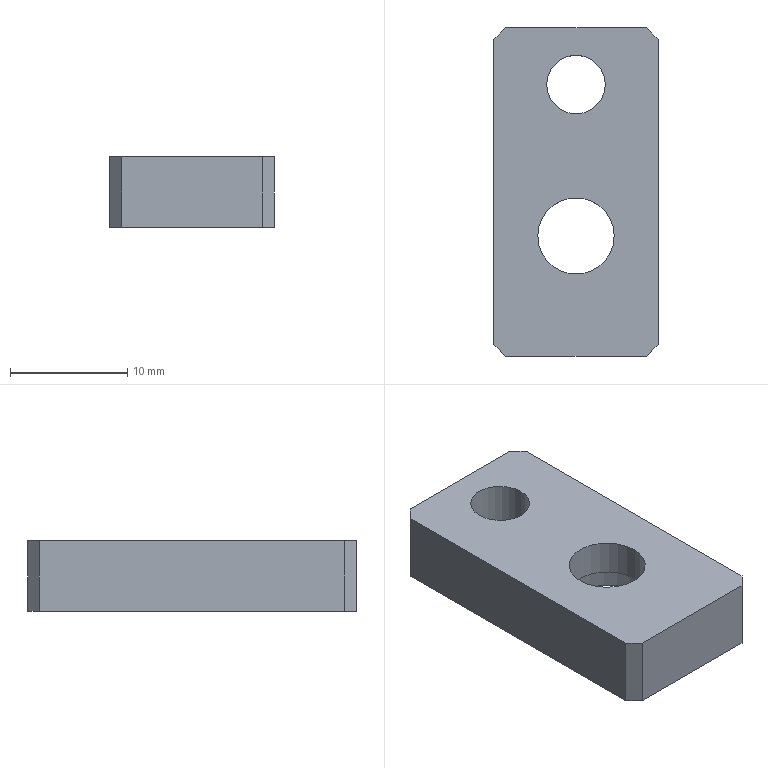Part | STEP file | Front Guide Wheel Fixing Plate | 1 solid | 17 faces | box 14 x 28 x 6 mm | volume 1838 mm3 | plane 11 | cylinder 6 | commonest cylinder face diameters 5 x2 6.5 x2 11 x2
STEP:
#1=CARTESIAN_POINT('',(0.,0.,0.));
#2=DIRECTION('',(0.,0.,1.));
#3=DIRECTION('',(1.,0.,0.));
#4=AXIS2_PLACEMENT_3D('',#1,#2,#3);
#5=CARTESIAN_POINT('',(-5.5,-2.25,3.));
#6=VERTEX_POINT('',#5);
#7=CARTESIAN_POINT('',(-5.5,-2.25,0.));
#8=VERTEX_POINT('',#7);
#9=CARTESIAN_POINT('',(-5.5,-2.25,0.));
#10=DIRECTION('',(0.,0.,-1.));
#11=VECTOR('',#10,1.);
#12=LINE('',#9,#11);
#13=CARTESIAN_POINT('',(0.,-2.25,0.));
#14=DIRECTION('',(0.,0.,-1.));
#15=DIRECTION('',(-1.,0.,0.));
#16=AXIS2_PLACEMENT_3D('',#13,#14,#15);
#17=CYLINDRICAL_SURFACE('',#16,5.5);
#18=CARTESIAN_POINT('',(6.283,0.));
#19=DIRECTION('',(0.,1.));
#20=VECTOR('',#19,1.);
#21=LINE('',#18,#20);
#22=(GEOMETRIC_REPRESENTATION_CONTEXT(2)PARAMETRIC_REPRESENTATION_CONTEXT()REPRESENTATION_CONTEXT('',''));
#23=DEFINITIONAL_REPRESENTATION('',(#21),#22);
#24=PCURVE('',#17,#23);
#25=CARTESIAN_POINT('',(0.,-2.25,0.));
#26=DIRECTION('',(0.,0.,-1.));
#27=DIRECTION('',(-1.,0.,0.));
#28=AXIS2_PLACEMENT_3D('',#25,#26,#27);
#29=CYLINDRICAL_SURFACE('',#28,5.5);
#30=CARTESIAN_POINT('',(0.,0.));
#31=DIRECTION('',(0.,1.));
#32=VECTOR('',#31,1.);
#33=LINE('',#30,#32);
#34=(GEOMETRIC_REPRESENTATION_CONTEXT(2)PARAMETRIC_REPRESENTATION_CONTEXT()REPRESENTATION_CONTEXT('',''));
#35=DEFINITIONAL_REPRESENTATION('',(#33),#34);
#36=PCURVE('',#29,#35);
#37=SURFACE_CURVE('',#12,(#24,#36),.PCURVE_S1.);
#38=EDGE_CURVE('',#6,#8,#37,.T.);
#39=ORIENTED_EDGE('',*,*,#38,.T.);
#40=CARTESIAN_POINT('',(5.5,-2.25,0.));
#41=VERTEX_POINT('',#40);
#42=CARTESIAN_POINT('',(0.,-2.25,0.));
#43=DIRECTION('',(0.,0.,-1.));
#44=DIRECTION('',(-1.,0.,0.));
#45=AXIS2_PLACEMENT_3D('',#42,#43,#44);
#46=CIRCLE('',#45,5.5);
#47=CARTESIAN_POINT('',(0.,0.));
#48=DIRECTION('',(1.,0.));
#49=VECTOR('',#48,1.);
#50=LINE('',#47,#49);
#51=(GEOMETRIC_REPRESENTATION_CONTEXT(2)PARAMETRIC_REPRESENTATION_CONTEXT()REPRESENTATION_CONTEXT('',''));
#52=DEFINITIONAL_REPRESENTATION('',(#50),#51);
#53=PCURVE('',#17,#52);
#54=CARTESIAN_POINT('',(0.,0.,0.));
#55=DIRECTION('',(0.,0.,1.));
#56=DIRECTION('',(1.,0.,0.));
#57=AXIS2_PLACEMENT_3D('',#54,#55,#56);
#58=PLANE('',#57);
#59=CARTESIAN_POINT('',(-5.5,-2.25));
#60=CARTESIAN_POINT('',(-5.5,7.276));
#61=CARTESIAN_POINT('',(2.75,2.513));
#62=CARTESIAN_POINT('',(11.,-2.25));
#63=CARTESIAN_POINT('',(2.75,-7.013));
#64=CARTESIAN_POINT('',(-5.5,-11.776));
#65=CARTESIAN_POINT('',(-5.5,-2.25));
#66=(BOUNDED_CURVE()B_SPLINE_CURVE(2,(#59,#60,#61,#62,#63,#64,#65),.UNSPECIFIED.,.T.,.F.)B_SPLINE_CURVE_WITH_KNOTS((1,2,2,2,2,1),(-2.094,0.,2.094,4.189,6.283,8.378),.UNSPECIFIED.)CURVE()GEOMETRIC_REPRESENTATION_ITEM()RATIONAL_B_SPLINE_CURVE((1.,0.5,1.,0.5,1.,0.5,1.))REPRESENTATION_ITEM(''));
#67=(GEOMETRIC_REPRESENTATION_CONTEXT(2)PARAMETRIC_REPRESENTATION_CONTEXT()REPRESENTATION_CONTEXT('',''));
#68=DEFINITIONAL_REPRESENTATION('',(#66),#67);
#69=PCURVE('',#58,#68);
#70=SURFACE_CURVE('',#46,(#53,#69),.PCURVE_S1.);
#71=EDGE_CURVE('',#41,#8,#70,.T.);
#72=ORIENTED_EDGE('',*,*,#71,.F.);
#73=CARTESIAN_POINT('',(5.5,-2.25,3.));
#74=VERTEX_POINT('',#73);
#75=CARTESIAN_POINT('',(5.5,-2.25,0.));
#76=DIRECTION('',(0.,0.,-1.));
#77=VECTOR('',#76,1.);
#78=LINE('',#75,#77);
#79=CARTESIAN_POINT('',(3.142,0.));
#80=DIRECTION('',(0.,1.));
#81=VECTOR('',#80,1.);
#82=LINE('',#79,#81);
#83=(GEOMETRIC_REPRESENTATION_CONTEXT(2)PARAMETRIC_REPRESENTATION_CONTEXT()REPRESENTATION_CONTEXT('',''));
#84=DEFINITIONAL_REPRESENTATION('',(#82),#83);
#85=PCURVE('',#17,#84);
#86=CARTESIAN_POINT('',(3.142,0.));
#87=DIRECTION('',(0.,1.));
#88=VECTOR('',#87,1.);
#89=LINE('',#86,#88);
#90=(GEOMETRIC_REPRESENTATION_CONTEXT(2)PARAMETRIC_REPRESENTATION_CONTEXT()REPRESENTATION_CONTEXT('',''));
#91=DEFINITIONAL_REPRESENTATION('',(#89),#90);
#92=PCURVE('',#29,#91);
#93=SURFACE_CURVE('',#78,(#85,#92),.PCURVE_S1.);
#94=EDGE_CURVE('',#74,#41,#93,.T.);
#95=ORIENTED_EDGE('',*,*,#94,.F.);
#96=CARTESIAN_POINT('',(0.,-2.25,3.));
#97=DIRECTION('',(0.,0.,-1.));
#98=DIRECTION('',(-1.,0.,0.));
#99=AXIS2_PLACEMENT_3D('',#96,#97,#98);
#100=CIRCLE('',#99,5.5);
#101=CARTESIAN_POINT('',(0.,-3.));
#102=DIRECTION('',(1.,0.));
#103=VECTOR('',#102,1.);
#104=LINE('',#101,#103);
#105=(GEOMETRIC_REPRESENTATION_CONTEXT(2)PARAMETRIC_REPRESENTATION_CONTEXT()REPRESENTATION_CONTEXT('',''));
#106=DEFINITIONAL_REPRESENTATION('',(#104),#105);
#107=PCURVE('',#17,#106);
#108=CARTESIAN_POINT('',(3.25,-2.25,3.));
#109=DIRECTION('',(0.,0.,1.));
#110=DIRECTION('',(1.,0.,0.));
#111=AXIS2_PLACEMENT_3D('',#108,#109,#110);
#112=PLANE('',#111);
#113=CARTESIAN_POINT('',(-8.75,0.));
#114=CARTESIAN_POINT('',(-8.75,9.526));
#115=CARTESIAN_POINT('',(-0.5,4.763));
#116=CARTESIAN_POINT('',(7.75,0.));
#117=CARTESIAN_POINT('',(-0.5,-4.763));
#118=CARTESIAN_POINT('',(-8.75,-9.526));
#119=CARTESIAN_POINT('',(-8.75,0.));
#120=(BOUNDED_CURVE()B_SPLINE_CURVE(2,(#113,#114,#115,#116,#117,#118,#119),.UNSPECIFIED.,.T.,.F.)B_SPLINE_CURVE_WITH_KNOTS((1,2,2,2,2,1),(-2.094,0.,2.094,4.189,6.283,8.378),.UNSPECIFIED.)CURVE()GEOMETRIC_REPRESENTATION_ITEM()RATIONAL_B_SPLINE_CURVE((1.,0.5,1.,0.5,1.,0.5,1.))REPRESENTATION_ITEM(''));
#121=(GEOMETRIC_REPRESENTATION_CONTEXT(2)PARAMETRIC_REPRESENTATION_CONTEXT()REPRESENTATION_CONTEXT('',''));
#122=DEFINITIONAL_REPRESENTATION('',(#120),#121);
#123=PCURVE('',#112,#122);
#124=SURFACE_CURVE('',#100,(#107,#123),.PCURVE_S1.);
#125=EDGE_CURVE('',#74,#6,#124,.T.);
#126=ORIENTED_EDGE('',*,*,#125,.T.);
#127=EDGE_LOOP('',(#39,#72,#95,#126));
#128=FACE_BOUND('',#127,.F.);
#129=ADVANCED_FACE('',(#128),#17,.F.);
#130=CARTESIAN_POINT('',(-3.25,-2.25,6.));
#131=VERTEX_POINT('',#130);
#132=CARTESIAN_POINT('',(-3.25,-2.25,3.));
#133=VERTEX_POINT('',#132);
#134=CARTESIAN_POINT('',(-3.25,-2.25,0.));
#135=DIRECTION('',(0.,0.,-1.));
#136=VECTOR('',#135,1.);
#137=LINE('',#134,#136);
#138=CARTESIAN_POINT('',(0.,-2.25,0.));
#139=DIRECTION('',(0.,0.,-1.));
#140=DIRECTION('',(-1.,0.,0.));
#141=AXIS2_PLACEMENT_3D('',#138,#139,#140);
#142=CYLINDRICAL_SURFACE('',#141,3.25);
#143=CARTESIAN_POINT('',(6.283,0.));
#144=DIRECTION('',(0.,1.));
#145=VECTOR('',#144,1.);
#146=LINE('',#143,#145);
#147=(GEOMETRIC_REPRESENTATION_CONTEXT(2)PARAMETRIC_REPRESENTATION_CONTEXT()REPRESENTATION_CONTEXT('',''));
#148=DEFINITIONAL_REPRESENTATION('',(#146),#147);
#149=PCURVE('',#142,#148);
#150=CARTESIAN_POINT('',(0.,-2.25,0.));
#151=DIRECTION('',(0.,0.,-1.));
#152=DIRECTION('',(-1.,0.,0.));
#153=AXIS2_PLACEMENT_3D('',#150,#151,#152);
#154=CYLINDRICAL_SURFACE('',#153,3.25);
#155=CARTESIAN_POINT('',(0.,0.));
#156=DIRECTION('',(0.,1.));
#157=VECTOR('',#156,1.);
#158=LINE('',#155,#157);
#159=(GEOMETRIC_REPRESENTATION_CONTEXT(2)PARAMETRIC_REPRESENTATION_CONTEXT()REPRESENTATION_CONTEXT('',''));
#160=DEFINITIONAL_REPRESENTATION('',(#158),#159);
#161=PCURVE('',#154,#160);
#162=SURFACE_CURVE('',#137,(#149,#161),.PCURVE_S1.);
#163=EDGE_CURVE('',#131,#133,#162,.T.);
#164=ORIENTED_EDGE('',*,*,#163,.T.);
#165=CARTESIAN_POINT('',(3.25,-2.25,3.));
#166=VERTEX_POINT('',#165);
#167=CARTESIAN_POINT('',(0.,-2.25,3.));
#168=DIRECTION('',(0.,0.,-1.));
#169=DIRECTION('',(-1.,0.,0.));
#170=AXIS2_PLACEMENT_3D('',#167,#168,#169);
#171=CIRCLE('',#170,3.25);
#172=CARTESIAN_POINT('',(0.,-3.));
#173=DIRECTION('',(1.,0.));
#174=VECTOR('',#173,1.);
#175=LINE('',#172,#174);
#176=(GEOMETRIC_REPRESENTATION_CONTEXT(2)PARAMETRIC_REPRESENTATION_CONTEXT()REPRESENTATION_CONTEXT('',''));
#177=DEFINITIONAL_REPRESENTATION('',(#175),#176);
#178=PCURVE('',#142,#177);
#179=CARTESIAN_POINT('',(-6.5,0.));
#180=CARTESIAN_POINT('',(-6.5,5.629));
#181=CARTESIAN_POINT('',(-1.625,2.815));
#182=CARTESIAN_POINT('',(3.25,0.));
#183=CARTESIAN_POINT('',(-1.625,-2.815));
#184=CARTESIAN_POINT('',(-6.5,-5.629));
#185=CARTESIAN_POINT('',(-6.5,0.));
#186=(BOUNDED_CURVE()B_SPLINE_CURVE(2,(#179,#180,#181,#182,#183,#184,#185),.UNSPECIFIED.,.T.,.F.)B_SPLINE_CURVE_WITH_KNOTS((1,2,2,2,2,1),(-2.094,0.,2.094,4.189,6.283,8.378),.UNSPECIFIED.)CURVE()GEOMETRIC_REPRESENTATION_ITEM()RATIONAL_B_SPLINE_CURVE((1.,0.5,1.,0.5,1.,0.5,1.))REPRESENTATION_ITEM(''));
#187=(GEOMETRIC_REPRESENTATION_CONTEXT(2)PARAMETRIC_REPRESENTATION_CONTEXT()REPRESENTATION_CONTEXT('',''));
#188=DEFINITIONAL_REPRESENTATION('',(#186),#187);
#189=PCURVE('',#112,#188);
#190=SURFACE_CURVE('',#171,(#178,#189),.PCURVE_S1.);
#191=EDGE_CURVE('',#166,#133,#190,.T.);
#192=ORIENTED_EDGE('',*,*,#191,.F.);
#193=CARTESIAN_POINT('',(3.25,-2.25,6.));
#194=VERTEX_POINT('',#193);
#195=CARTESIAN_POINT('',(3.25,-2.25,0.));
#196=DIRECTION('',(0.,0.,-1.));
#197=VECTOR('',#196,1.);
#198=LINE('',#195,#197);
#199=CARTESIAN_POINT('',(3.142,0.));
#200=DIRECTION('',(0.,1.));
#201=VECTOR('',#200,1.);
#202=LINE('',#199,#201);
#203=(GEOMETRIC_REPRESENTATION_CONTEXT(2)PARAMETRIC_REPRESENTATION_CONTEXT()REPRESENTATION_CONTEXT('',''));
#204=DEFINITIONAL_REPRESENTATION('',(#202),#203);
#205=PCURVE('',#142,#204);
#206=CARTESIAN_POINT('',(3.142,0.));
#207=DIRECTION('',(0.,1.));
#208=VECTOR('',#207,1.);
#209=LINE('',#206,#208);
#210=(GEOMETRIC_REPRESENTATION_CONTEXT(2)PARAMETRIC_REPRESENTATION_CONTEXT()REPRESENTATION_CONTEXT('',''));
#211=DEFINITIONAL_REPRESENTATION('',(#209),#210);
#212=PCURVE('',#154,#211);
#213=SURFACE_CURVE('',#198,(#205,#212),.PCURVE_S1.);
#214=EDGE_CURVE('',#194,#166,#213,.T.);
#215=ORIENTED_EDGE('',*,*,#214,.F.);
#216=CARTESIAN_POINT('',(0.,-2.25,6.));
#217=DIRECTION('',(0.,0.,-1.));
#218=DIRECTION('',(-1.,0.,0.));
#219=AXIS2_PLACEMENT_3D('',#216,#217,#218);
#220=CIRCLE('',#219,3.25);
#221=CARTESIAN_POINT('',(0.,-6.));
#222=DIRECTION('',(1.,0.));
#223=VECTOR('',#222,1.);
#224=LINE('',#221,#223);
#225=(GEOMETRIC_REPRESENTATION_CONTEXT(2)PARAMETRIC_REPRESENTATION_CONTEXT()REPRESENTATION_CONTEXT('',''));
#226=DEFINITIONAL_REPRESENTATION('',(#224),#225);
#227=PCURVE('',#142,#226);
#228=CARTESIAN_POINT('',(0.,0.,6.));
#229=DIRECTION('',(0.,0.,1.));
#230=DIRECTION('',(1.,0.,0.));
#231=AXIS2_PLACEMENT_3D('',#228,#229,#230);
#232=PLANE('',#231);
#233=CARTESIAN_POINT('',(-3.25,-2.25));
#234=CARTESIAN_POINT('',(-3.25,3.379));
#235=CARTESIAN_POINT('',(1.625,0.5646));
#236=CARTESIAN_POINT('',(6.5,-2.25));
#237=CARTESIAN_POINT('',(1.625,-5.065));
#238=CARTESIAN_POINT('',(-3.25,-7.879));
#239=CARTESIAN_POINT('',(-3.25,-2.25));
#240=(BOUNDED_CURVE()B_SPLINE_CURVE(2,(#233,#234,#235,#236,#237,#238,#239),.UNSPECIFIED.,.T.,.F.)B_SPLINE_CURVE_WITH_KNOTS((1,2,2,2,2,1),(-2.094,0.,2.094,4.189,6.283,8.378),.UNSPECIFIED.)CURVE()GEOMETRIC_REPRESENTATION_ITEM()RATIONAL_B_SPLINE_CURVE((1.,0.5,1.,0.5,1.,0.5,1.))REPRESENTATION_ITEM(''));
#241=(GEOMETRIC_REPRESENTATION_CONTEXT(2)PARAMETRIC_REPRESENTATION_CONTEXT()REPRESENTATION_CONTEXT('',''));
#242=DEFINITIONAL_REPRESENTATION('',(#240),#241);
#243=PCURVE('',#232,#242);
#244=SURFACE_CURVE('',#220,(#227,#243),.PCURVE_S1.);
#245=EDGE_CURVE('',#194,#131,#244,.T.);
#246=ORIENTED_EDGE('',*,*,#245,.T.);
#247=EDGE_LOOP('',(#164,#192,#215,#246));
#248=FACE_BOUND('',#247,.F.);
#249=ADVANCED_FACE('',(#248),#142,.F.);
#250=CARTESIAN_POINT('',(-2.5,10.65,6.));
#251=VERTEX_POINT('',#250);
#252=CARTESIAN_POINT('',(-2.5,10.65,0.));
#253=VERTEX_POINT('',#252);
#254=CARTESIAN_POINT('',(-2.5,10.65,6.));
#255=DIRECTION('',(0.,0.,-1.));
#256=VECTOR('',#255,1.);
#257=LINE('',#254,#256);
#258=CARTESIAN_POINT('',(0.,10.65,6.));
#259=DIRECTION('',(0.,0.,-1.));
#260=DIRECTION('',(-1.,0.,0.));
#261=AXIS2_PLACEMENT_3D('',#258,#259,#260);
#262=CYLINDRICAL_SURFACE('',#261,2.5);
#263=CARTESIAN_POINT('',(6.283,0.));
#264=DIRECTION('',(0.,1.));
#265=VECTOR('',#264,1.);
#266=LINE('',#263,#265);
#267=(GEOMETRIC_REPRESENTATION_CONTEXT(2)PARAMETRIC_REPRESENTATION_CONTEXT()REPRESENTATION_CONTEXT('',''));
#268=DEFINITIONAL_REPRESENTATION('',(#266),#267);
#269=PCURVE('',#262,#268);
#270=CARTESIAN_POINT('',(0.,10.65,6.));
#271=DIRECTION('',(0.,0.,-1.));
#272=DIRECTION('',(-1.,0.,0.));
#273=AXIS2_PLACEMENT_3D('',#270,#271,#272);
#274=CYLINDRICAL_SURFACE('',#273,2.5);
#275=CARTESIAN_POINT('',(0.,0.));
#276=DIRECTION('',(0.,1.));
#277=VECTOR('',#276,1.);
#278=LINE('',#275,#277);
#279=(GEOMETRIC_REPRESENTATION_CONTEXT(2)PARAMETRIC_REPRESENTATION_CONTEXT()REPRESENTATION_CONTEXT('',''));
#280=DEFINITIONAL_REPRESENTATION('',(#278),#279);
#281=PCURVE('',#274,#280);
#282=SURFACE_CURVE('',#257,(#269,#281),.PCURVE_S1.);
#283=EDGE_CURVE('',#251,#253,#282,.T.);
#284=ORIENTED_EDGE('',*,*,#283,.T.);
#285=CARTESIAN_POINT('',(2.5,10.65,0.));
#286=VERTEX_POINT('',#285);
#287=CARTESIAN_POINT('',(0.,10.65,0.));
#288=DIRECTION('',(0.,0.,1.));
#289=DIRECTION('',(1.,0.,0.));
#290=AXIS2_PLACEMENT_3D('',#287,#288,#289);
#291=CIRCLE('',#290,2.5);
#292=CARTESIAN_POINT('',(9.425,6.));
#293=DIRECTION('',(-1.,0.));
#294=VECTOR('',#293,1.);
#295=LINE('',#292,#294);
#296=(GEOMETRIC_REPRESENTATION_CONTEXT(2)PARAMETRIC_REPRESENTATION_CONTEXT()REPRESENTATION_CONTEXT('',''));
#297=DEFINITIONAL_REPRESENTATION('',(#295),#296);
#298=PCURVE('',#262,#297);
#299=CARTESIAN_POINT('',(0.,10.65));
#300=DIRECTION('',(1.,0.));
#301=AXIS2_PLACEMENT_2D('',#299,#300);
#302=CIRCLE('',#301,2.5);
#303=(GEOMETRIC_REPRESENTATION_CONTEXT(2)PARAMETRIC_REPRESENTATION_CONTEXT()REPRESENTATION_CONTEXT('',''));
#304=DEFINITIONAL_REPRESENTATION('',(#302),#303);
#305=PCURVE('',#58,#304);
#306=SURFACE_CURVE('',#291,(#298,#305),.PCURVE_S1.);
#307=EDGE_CURVE('',#253,#286,#306,.T.);
#308=ORIENTED_EDGE('',*,*,#307,.T.);
#309=CARTESIAN_POINT('',(2.5,10.65,6.));
#310=VERTEX_POINT('',#309);
#311=CARTESIAN_POINT('',(2.5,10.65,6.));
#312=DIRECTION('',(0.,0.,-1.));
#313=VECTOR('',#312,1.);
#314=LINE('',#311,#313);
#315=CARTESIAN_POINT('',(3.142,0.));
#316=DIRECTION('',(0.,1.));
#317=VECTOR('',#316,1.);
#318=LINE('',#315,#317);
#319=(GEOMETRIC_REPRESENTATION_CONTEXT(2)PARAMETRIC_REPRESENTATION_CONTEXT()REPRESENTATION_CONTEXT('',''));
#320=DEFINITIONAL_REPRESENTATION('',(#318),#319);
#321=PCURVE('',#262,#320);
#322=CARTESIAN_POINT('',(3.142,0.));
#323=DIRECTION('',(0.,1.));
#324=VECTOR('',#323,1.);
#325=LINE('',#322,#324);
#326=(GEOMETRIC_REPRESENTATION_CONTEXT(2)PARAMETRIC_REPRESENTATION_CONTEXT()REPRESENTATION_CONTEXT('',''));
#327=DEFINITIONAL_REPRESENTATION('',(#325),#326);
#328=PCURVE('',#274,#327);
#329=SURFACE_CURVE('',#314,(#321,#328),.PCURVE_S1.);
#330=EDGE_CURVE('',#310,#286,#329,.T.);
#331=ORIENTED_EDGE('',*,*,#330,.F.);
#332=CARTESIAN_POINT('',(0.,10.65,6.));
#333=DIRECTION('',(0.,0.,1.));
#334=DIRECTION('',(1.,0.,0.));
#335=AXIS2_PLACEMENT_3D('',#332,#333,#334);
#336=CIRCLE('',#335,2.5);
#337=CARTESIAN_POINT('',(9.425,0.));
#338=DIRECTION('',(-1.,0.));
#339=VECTOR('',#338,1.);
#340=LINE('',#337,#339);
#341=(GEOMETRIC_REPRESENTATION_CONTEXT(2)PARAMETRIC_REPRESENTATION_CONTEXT()REPRESENTATION_CONTEXT('',''));
#342=DEFINITIONAL_REPRESENTATION('',(#340),#341);
#343=PCURVE('',#262,#342);
#344=CARTESIAN_POINT('',(0.,10.65));
#345=DIRECTION('',(1.,0.));
#346=AXIS2_PLACEMENT_2D('',#344,#345);
#347=CIRCLE('',#346,2.5);
#348=(GEOMETRIC_REPRESENTATION_CONTEXT(2)PARAMETRIC_REPRESENTATION_CONTEXT()REPRESENTATION_CONTEXT('',''));
#349=DEFINITIONAL_REPRESENTATION('',(#347),#348);
#350=PCURVE('',#232,#349);
#351=SURFACE_CURVE('',#336,(#343,#350),.PCURVE_S1.);
#352=EDGE_CURVE('',#251,#310,#351,.T.);
#353=ORIENTED_EDGE('',*,*,#352,.F.);
#354=EDGE_LOOP('',(#284,#308,#331,#353));
#355=FACE_BOUND('',#354,.F.);
#356=ADVANCED_FACE('',(#355),#262,.F.);
#357=CARTESIAN_POINT('',(0.,-2.25,6.));
#358=DIRECTION('',(0.,0.,-1.));
#359=DIRECTION('',(-1.,0.,0.));
#360=AXIS2_PLACEMENT_3D('',#357,#358,#359);
#361=CIRCLE('',#360,3.25);
#362=CARTESIAN_POINT('',(-3.25,-2.25));
#363=CARTESIAN_POINT('',(-3.25,3.379));
#364=CARTESIAN_POINT('',(1.625,0.5646));
#365=CARTESIAN_POINT('',(6.5,-2.25));
#366=CARTESIAN_POINT('',(1.625,-5.065));
#367=CARTESIAN_POINT('',(-3.25,-7.879));
#368=CARTESIAN_POINT('',(-3.25,-2.25));
#369=(BOUNDED_CURVE()B_SPLINE_CURVE(2,(#362,#363,#364,#365,#366,#367,#368),.UNSPECIFIED.,.T.,.F.)B_SPLINE_CURVE_WITH_KNOTS((1,2,2,2,2,1),(-2.094,0.,2.094,4.189,6.283,8.378),.UNSPECIFIED.)CURVE()GEOMETRIC_REPRESENTATION_ITEM()RATIONAL_B_SPLINE_CURVE((1.,0.5,1.,0.5,1.,0.5,1.))REPRESENTATION_ITEM(''));
#370=(GEOMETRIC_REPRESENTATION_CONTEXT(2)PARAMETRIC_REPRESENTATION_CONTEXT()REPRESENTATION_CONTEXT('',''));
#371=DEFINITIONAL_REPRESENTATION('',(#369),#370);
#372=PCURVE('',#232,#371);
#373=CARTESIAN_POINT('',(0.,-6.));
#374=DIRECTION('',(1.,0.));
#375=VECTOR('',#374,1.);
#376=LINE('',#373,#375);
#377=(GEOMETRIC_REPRESENTATION_CONTEXT(2)PARAMETRIC_REPRESENTATION_CONTEXT()REPRESENTATION_CONTEXT('',''));
#378=DEFINITIONAL_REPRESENTATION('',(#376),#377);
#379=PCURVE('',#154,#378);
#380=SURFACE_CURVE('',#361,(#372,#379),.PCURVE_S1.);
#381=EDGE_CURVE('',#131,#194,#380,.T.);
#382=ORIENTED_EDGE('',*,*,#381,.T.);
#383=ORIENTED_EDGE('',*,*,#245,.T.);
#384=EDGE_LOOP('',(#382,#383));
#385=FACE_BOUND('',#384,.T.);
#386=CARTESIAN_POINT('',(-6.,-12.5,6.));
#387=VERTEX_POINT('',#386);
#388=CARTESIAN_POINT('',(6.,-12.5,6.));
#389=VERTEX_POINT('',#388);
#390=CARTESIAN_POINT('',(-7.,-12.5,6.));
#391=DIRECTION('',(1.,0.,0.));
#392=VECTOR('',#391,1.);
#393=LINE('',#390,#392);
#394=CARTESIAN_POINT('',(-7.,-12.5));
#395=DIRECTION('',(1.,0.));
#396=VECTOR('',#395,1.);
#397=LINE('',#394,#396);
#398=(GEOMETRIC_REPRESENTATION_CONTEXT(2)PARAMETRIC_REPRESENTATION_CONTEXT()REPRESENTATION_CONTEXT('',''));
#399=DEFINITIONAL_REPRESENTATION('',(#397),#398);
#400=PCURVE('',#232,#399);
#401=CARTESIAN_POINT('',(-7.,-12.5,6.));
#402=DIRECTION('',(0.,1.,0.));
#403=DIRECTION('',(-1.,0.,0.));
#404=AXIS2_PLACEMENT_3D('',#401,#402,#403);
#405=PLANE('',#404);
#406=CARTESIAN_POINT('',(0.,0.));
#407=DIRECTION('',(-1.,0.));
#408=VECTOR('',#407,1.);
#409=LINE('',#406,#408);
#410=(GEOMETRIC_REPRESENTATION_CONTEXT(2)PARAMETRIC_REPRESENTATION_CONTEXT()REPRESENTATION_CONTEXT('',''));
#411=DEFINITIONAL_REPRESENTATION('',(#409),#410);
#412=PCURVE('',#405,#411);
#413=SURFACE_CURVE('',#393,(#400,#412),.PCURVE_S1.);
#414=EDGE_CURVE('',#387,#389,#413,.T.);
#415=ORIENTED_EDGE('',*,*,#414,.T.);
#416=CARTESIAN_POINT('',(7.,-11.5,6.));
#417=VERTEX_POINT('',#416);
#418=CARTESIAN_POINT('',(9.25,-9.25,6.));
#419=DIRECTION('',(0.7071,0.7071,0.));
#420=VECTOR('',#419,1.);
#421=LINE('',#418,#420);
#422=CARTESIAN_POINT('',(9.25,-9.25));
#423=DIRECTION('',(0.7071,0.7071));
#424=VECTOR('',#423,1.);
#425=LINE('',#422,#424);
#426=(GEOMETRIC_REPRESENTATION_CONTEXT(2)PARAMETRIC_REPRESENTATION_CONTEXT()REPRESENTATION_CONTEXT('',''));
#427=DEFINITIONAL_REPRESENTATION('',(#425),#426);
#428=PCURVE('',#232,#427);
#429=CARTESIAN_POINT('',(7.,-11.5,6.));
#430=DIRECTION('',(-0.7071,0.7071,0.));
#431=DIRECTION('',(0.,0.,-1.));
#432=AXIS2_PLACEMENT_3D('',#429,#430,#431);
#433=PLANE('',#432);
#434=CARTESIAN_POINT('',(0.,-3.182));
#435=DIRECTION('',(0.,-1.));
#436=VECTOR('',#435,1.);
#437=LINE('',#434,#436);
#438=(GEOMETRIC_REPRESENTATION_CONTEXT(2)PARAMETRIC_REPRESENTATION_CONTEXT()REPRESENTATION_CONTEXT('',''));
#439=DEFINITIONAL_REPRESENTATION('',(#437),#438);
#440=PCURVE('',#433,#439);
#441=SURFACE_CURVE('',#421,(#428,#440),.PCURVE_S1.);
#442=EDGE_CURVE('',#389,#417,#441,.T.);
#443=ORIENTED_EDGE('',*,*,#442,.T.);
#444=CARTESIAN_POINT('',(7.,14.5,6.));
#445=VERTEX_POINT('',#444);
#446=CARTESIAN_POINT('',(7.,15.5,6.));
#447=DIRECTION('',(0.,1.,0.));
#448=VECTOR('',#447,1.);
#449=LINE('',#446,#448);
#450=CARTESIAN_POINT('',(7.,15.5));
#451=DIRECTION('',(0.,1.));
#452=VECTOR('',#451,1.);
#453=LINE('',#450,#452);
#454=(GEOMETRIC_REPRESENTATION_CONTEXT(2)PARAMETRIC_REPRESENTATION_CONTEXT()REPRESENTATION_CONTEXT('',''));
#455=DEFINITIONAL_REPRESENTATION('',(#453),#454);
#456=PCURVE('',#232,#455);
#457=CARTESIAN_POINT('',(7.,15.5,6.));
#458=DIRECTION('',(-1.,0.,0.));
#459=DIRECTION('',(0.,-1.,0.));
#460=AXIS2_PLACEMENT_3D('',#457,#458,#459);
#461=PLANE('',#460);
#462=CARTESIAN_POINT('',(0.,0.));
#463=DIRECTION('',(-1.,0.));
#464=VECTOR('',#463,1.);
#465=LINE('',#462,#464);
#466=(GEOMETRIC_REPRESENTATION_CONTEXT(2)PARAMETRIC_REPRESENTATION_CONTEXT()REPRESENTATION_CONTEXT('',''));
#467=DEFINITIONAL_REPRESENTATION('',(#465),#466);
#468=PCURVE('',#461,#467);
#469=SURFACE_CURVE('',#449,(#456,#468),.PCURVE_S1.);
#470=EDGE_CURVE('',#417,#445,#469,.T.);
#471=ORIENTED_EDGE('',*,*,#470,.T.);
#472=CARTESIAN_POINT('',(6.,15.5,6.));
#473=VERTEX_POINT('',#472);
#474=CARTESIAN_POINT('',(10.75,10.75,6.));
#475=DIRECTION('',(-0.7071,0.7071,0.));
#476=VECTOR('',#475,1.);
#477=LINE('',#474,#476);
#478=CARTESIAN_POINT('',(10.75,10.75));
#479=DIRECTION('',(-0.7071,0.7071));
#480=VECTOR('',#479,1.);
#481=LINE('',#478,#480);
#482=(GEOMETRIC_REPRESENTATION_CONTEXT(2)PARAMETRIC_REPRESENTATION_CONTEXT()REPRESENTATION_CONTEXT('',''));
#483=DEFINITIONAL_REPRESENTATION('',(#481),#482);
#484=PCURVE('',#232,#483);
#485=CARTESIAN_POINT('',(6.,15.5,6.));
#486=DIRECTION('',(-0.7071,-0.7071,0.));
#487=DIRECTION('',(0.,0.,-1.));
#488=AXIS2_PLACEMENT_3D('',#485,#486,#487);
#489=PLANE('',#488);
#490=CARTESIAN_POINT('',(0.,6.718));
#491=DIRECTION('',(0.,-1.));
#492=VECTOR('',#491,1.);
#493=LINE('',#490,#492);
#494=(GEOMETRIC_REPRESENTATION_CONTEXT(2)PARAMETRIC_REPRESENTATION_CONTEXT()REPRESENTATION_CONTEXT('',''));
#495=DEFINITIONAL_REPRESENTATION('',(#493),#494);
#496=PCURVE('',#489,#495);
#497=SURFACE_CURVE('',#477,(#484,#496),.PCURVE_S1.);
#498=EDGE_CURVE('',#445,#473,#497,.T.);
#499=ORIENTED_EDGE('',*,*,#498,.T.);
#500=CARTESIAN_POINT('',(-6.,15.5,6.));
#501=VERTEX_POINT('',#500);
#502=CARTESIAN_POINT('',(-7.,15.5,6.));
#503=DIRECTION('',(-1.,0.,0.));
#504=VECTOR('',#503,1.);
#505=LINE('',#502,#504);
#506=CARTESIAN_POINT('',(-7.,15.5));
#507=DIRECTION('',(-1.,0.));
#508=VECTOR('',#507,1.);
#509=LINE('',#506,#508);
#510=(GEOMETRIC_REPRESENTATION_CONTEXT(2)PARAMETRIC_REPRESENTATION_CONTEXT()REPRESENTATION_CONTEXT('',''));
#511=DEFINITIONAL_REPRESENTATION('',(#509),#510);
#512=PCURVE('',#232,#511);
#513=CARTESIAN_POINT('',(-7.,15.5,6.));
#514=DIRECTION('',(0.,-1.,0.));
#515=DIRECTION('',(0.,0.,-1.));
#516=AXIS2_PLACEMENT_3D('',#513,#514,#515);
#517=PLANE('',#516);
#518=CARTESIAN_POINT('',(0.,0.));
#519=DIRECTION('',(0.,-1.));
#520=VECTOR('',#519,1.);
#521=LINE('',#518,#520);
#522=(GEOMETRIC_REPRESENTATION_CONTEXT(2)PARAMETRIC_REPRESENTATION_CONTEXT()REPRESENTATION_CONTEXT('',''));
#523=DEFINITIONAL_REPRESENTATION('',(#521),#522);
#524=PCURVE('',#517,#523);
#525=SURFACE_CURVE('',#505,(#512,#524),.PCURVE_S1.);
#526=EDGE_CURVE('',#473,#501,#525,.T.);
#527=ORIENTED_EDGE('',*,*,#526,.T.);
#528=CARTESIAN_POINT('',(-7.,14.5,6.));
#529=VERTEX_POINT('',#528);
#530=CARTESIAN_POINT('',(-10.75,10.75,6.));
#531=DIRECTION('',(-0.7071,-0.7071,0.));
#532=VECTOR('',#531,1.);
#533=LINE('',#530,#532);
#534=CARTESIAN_POINT('',(-10.75,10.75));
#535=DIRECTION('',(-0.7071,-0.7071));
#536=VECTOR('',#535,1.);
#537=LINE('',#534,#536);
#538=(GEOMETRIC_REPRESENTATION_CONTEXT(2)PARAMETRIC_REPRESENTATION_CONTEXT()REPRESENTATION_CONTEXT('',''));
#539=DEFINITIONAL_REPRESENTATION('',(#537),#538);
#540=PCURVE('',#232,#539);
#541=CARTESIAN_POINT('',(-7.,14.5,6.));
#542=DIRECTION('',(0.7071,-0.7071,0.));
#543=DIRECTION('',(0.,0.,-1.));
#544=AXIS2_PLACEMENT_3D('',#541,#542,#543);
#545=PLANE('',#544);
#546=CARTESIAN_POINT('',(0.,-5.303));
#547=DIRECTION('',(0.,-1.));
#548=VECTOR('',#547,1.);
#549=LINE('',#546,#548);
#550=(GEOMETRIC_REPRESENTATION_CONTEXT(2)PARAMETRIC_REPRESENTATION_CONTEXT()REPRESENTATION_CONTEXT('',''));
#551=DEFINITIONAL_REPRESENTATION('',(#549),#550);
#552=PCURVE('',#545,#551);
#553=SURFACE_CURVE('',#533,(#540,#552),.PCURVE_S1.);
#554=EDGE_CURVE('',#501,#529,#553,.T.);
#555=ORIENTED_EDGE('',*,*,#554,.T.);
#556=CARTESIAN_POINT('',(-7.,-11.5,6.));
#557=VERTEX_POINT('',#556);
#558=CARTESIAN_POINT('',(-7.,15.5,6.));
#559=DIRECTION('',(0.,-1.,0.));
#560=VECTOR('',#559,1.);
#561=LINE('',#558,#560);
#562=CARTESIAN_POINT('',(-7.,15.5));
#563=DIRECTION('',(0.,-1.));
#564=VECTOR('',#563,1.);
#565=LINE('',#562,#564);
#566=(GEOMETRIC_REPRESENTATION_CONTEXT(2)PARAMETRIC_REPRESENTATION_CONTEXT()REPRESENTATION_CONTEXT('',''));
#567=DEFINITIONAL_REPRESENTATION('',(#565),#566);
#568=PCURVE('',#232,#567);
#569=CARTESIAN_POINT('',(-7.,15.5,6.));
#570=DIRECTION('',(1.,0.,0.));
#571=DIRECTION('',(0.,1.,0.));
#572=AXIS2_PLACEMENT_3D('',#569,#570,#571);
#573=PLANE('',#572);
#574=CARTESIAN_POINT('',(0.,0.));
#575=DIRECTION('',(-1.,0.));
#576=VECTOR('',#575,1.);
#577=LINE('',#574,#576);
#578=(GEOMETRIC_REPRESENTATION_CONTEXT(2)PARAMETRIC_REPRESENTATION_CONTEXT()REPRESENTATION_CONTEXT('',''));
#579=DEFINITIONAL_REPRESENTATION('',(#577),#578);
#580=PCURVE('',#573,#579);
#581=SURFACE_CURVE('',#561,(#568,#580),.PCURVE_S1.);
#582=EDGE_CURVE('',#529,#557,#581,.T.);
#583=ORIENTED_EDGE('',*,*,#582,.T.);
#584=CARTESIAN_POINT('',(-9.25,-9.25,6.));
#585=DIRECTION('',(0.7071,-0.7071,0.));
#586=VECTOR('',#585,1.);
#587=LINE('',#584,#586);
#588=CARTESIAN_POINT('',(-9.25,-9.25));
#589=DIRECTION('',(0.7071,-0.7071));
#590=VECTOR('',#589,1.);
#591=LINE('',#588,#590);
#592=(GEOMETRIC_REPRESENTATION_CONTEXT(2)PARAMETRIC_REPRESENTATION_CONTEXT()REPRESENTATION_CONTEXT('',''));
#593=DEFINITIONAL_REPRESENTATION('',(#591),#592);
#594=PCURVE('',#232,#593);
#595=CARTESIAN_POINT('',(-6.,-12.5,6.));
#596=DIRECTION('',(0.7071,0.7071,0.));
#597=DIRECTION('',(0.,0.,-1.));
#598=AXIS2_PLACEMENT_3D('',#595,#596,#597);
#599=PLANE('',#598);
#600=CARTESIAN_POINT('',(0.,4.596));
#601=DIRECTION('',(0.,-1.));
#602=VECTOR('',#601,1.);
#603=LINE('',#600,#602);
#604=(GEOMETRIC_REPRESENTATION_CONTEXT(2)PARAMETRIC_REPRESENTATION_CONTEXT()REPRESENTATION_CONTEXT('',''));
#605=DEFINITIONAL_REPRESENTATION('',(#603),#604);
#606=PCURVE('',#599,#605);
#607=SURFACE_CURVE('',#587,(#594,#606),.PCURVE_S1.);
#608=EDGE_CURVE('',#557,#387,#607,.T.);
#609=ORIENTED_EDGE('',*,*,#608,.T.);
#610=EDGE_LOOP('',(#415,#443,#471,#499,#527,#555,#583,#609));
#611=FACE_BOUND('',#610,.T.);
#612=ORIENTED_EDGE('',*,*,#352,.F.);
#613=CARTESIAN_POINT('',(0.,10.65,6.));
#614=DIRECTION('',(0.,0.,1.));
#615=DIRECTION('',(1.,0.,0.));
#616=AXIS2_PLACEMENT_3D('',#613,#614,#615);
#617=CIRCLE('',#616,2.5);
#618=CARTESIAN_POINT('',(0.,10.65));
#619=DIRECTION('',(1.,0.));
#620=AXIS2_PLACEMENT_2D('',#618,#619);
#621=CIRCLE('',#620,2.5);
#622=(GEOMETRIC_REPRESENTATION_CONTEXT(2)PARAMETRIC_REPRESENTATION_CONTEXT()REPRESENTATION_CONTEXT('',''));
#623=DEFINITIONAL_REPRESENTATION('',(#621),#622);
#624=PCURVE('',#232,#623);
#625=CARTESIAN_POINT('',(3.142,0.));
#626=DIRECTION('',(-1.,0.));
#627=VECTOR('',#626,1.);
#628=LINE('',#625,#627);
#629=(GEOMETRIC_REPRESENTATION_CONTEXT(2)PARAMETRIC_REPRESENTATION_CONTEXT()REPRESENTATION_CONTEXT('',''));
#630=DEFINITIONAL_REPRESENTATION('',(#628),#629);
#631=PCURVE('',#274,#630);
#632=SURFACE_CURVE('',#617,(#624,#631),.PCURVE_S1.);
#633=EDGE_CURVE('',#310,#251,#632,.T.);
#634=ORIENTED_EDGE('',*,*,#633,.F.);
#635=EDGE_LOOP('',(#612,#634));
#636=FACE_BOUND('',#635,.T.);
#637=ADVANCED_FACE('',(#385,#611,#636),#232,.T.);
#638=CARTESIAN_POINT('',(0.,-2.25,0.));
#639=DIRECTION('',(0.,0.,-1.));
#640=DIRECTION('',(-1.,0.,0.));
#641=AXIS2_PLACEMENT_3D('',#638,#639,#640);
#642=CIRCLE('',#641,5.5);
#643=CARTESIAN_POINT('',(-5.5,-2.25));
#644=CARTESIAN_POINT('',(-5.5,7.276));
#645=CARTESIAN_POINT('',(2.75,2.513));
#646=CARTESIAN_POINT('',(11.,-2.25));
#647=CARTESIAN_POINT('',(2.75,-7.013));
#648=CARTESIAN_POINT('',(-5.5,-11.776));
#649=CARTESIAN_POINT('',(-5.5,-2.25));
#650=(BOUNDED_CURVE()B_SPLINE_CURVE(2,(#643,#644,#645,#646,#647,#648,#649),.UNSPECIFIED.,.T.,.F.)B_SPLINE_CURVE_WITH_KNOTS((1,2,2,2,2,1),(-2.094,0.,2.094,4.189,6.283,8.378),.UNSPECIFIED.)CURVE()GEOMETRIC_REPRESENTATION_ITEM()RATIONAL_B_SPLINE_CURVE((1.,0.5,1.,0.5,1.,0.5,1.))REPRESENTATION_ITEM(''));
#651=(GEOMETRIC_REPRESENTATION_CONTEXT(2)PARAMETRIC_REPRESENTATION_CONTEXT()REPRESENTATION_CONTEXT('',''));
#652=DEFINITIONAL_REPRESENTATION('',(#650),#651);
#653=PCURVE('',#58,#652);
#654=CARTESIAN_POINT('',(0.,0.));
#655=DIRECTION('',(1.,0.));
#656=VECTOR('',#655,1.);
#657=LINE('',#654,#656);
#658=(GEOMETRIC_REPRESENTATION_CONTEXT(2)PARAMETRIC_REPRESENTATION_CONTEXT()REPRESENTATION_CONTEXT('',''));
#659=DEFINITIONAL_REPRESENTATION('',(#657),#658);
#660=PCURVE('',#29,#659);
#661=SURFACE_CURVE('',#642,(#653,#660),.PCURVE_S1.);
#662=EDGE_CURVE('',#8,#41,#661,.T.);
#663=ORIENTED_EDGE('',*,*,#662,.F.);
#664=ORIENTED_EDGE('',*,*,#71,.F.);
#665=EDGE_LOOP('',(#663,#664));
#666=FACE_BOUND('',#665,.T.);
#667=CARTESIAN_POINT('',(7.,-11.5,0.));
#668=VERTEX_POINT('',#667);
#669=CARTESIAN_POINT('',(7.,14.5,0.));
#670=VERTEX_POINT('',#669);
#671=CARTESIAN_POINT('',(7.,15.5,0.));
#672=DIRECTION('',(0.,1.,0.));
#673=VECTOR('',#672,1.);
#674=LINE('',#671,#673);
#675=CARTESIAN_POINT('',(7.,15.5));
#676=DIRECTION('',(0.,1.));
#677=VECTOR('',#676,1.);
#678=LINE('',#675,#677);
#679=(GEOMETRIC_REPRESENTATION_CONTEXT(2)PARAMETRIC_REPRESENTATION_CONTEXT()REPRESENTATION_CONTEXT('',''));
#680=DEFINITIONAL_REPRESENTATION('',(#678),#679);
#681=PCURVE('',#58,#680);
#682=CARTESIAN_POINT('',(0.,-6.));
#683=DIRECTION('',(-1.,0.));
#684=VECTOR('',#683,1.);
#685=LINE('',#682,#684);
#686=(GEOMETRIC_REPRESENTATION_CONTEXT(2)PARAMETRIC_REPRESENTATION_CONTEXT()REPRESENTATION_CONTEXT('',''));
#687=DEFINITIONAL_REPRESENTATION('',(#685),#686);
#688=PCURVE('',#461,#687);
#689=SURFACE_CURVE('',#674,(#681,#688),.PCURVE_S1.);
#690=EDGE_CURVE('',#668,#670,#689,.T.);
#691=ORIENTED_EDGE('',*,*,#690,.F.);
#692=CARTESIAN_POINT('',(6.,-12.5,0.));
#693=VERTEX_POINT('',#692);
#694=CARTESIAN_POINT('',(7.,-11.5,0.));
#695=DIRECTION('',(-0.7071,-0.7071,0.));
#696=VECTOR('',#695,1.);
#697=LINE('',#694,#696);
#698=CARTESIAN_POINT('',(7.,-11.5));
#699=DIRECTION('',(-0.7071,-0.7071));
#700=VECTOR('',#699,1.);
#701=LINE('',#698,#700);
#702=(GEOMETRIC_REPRESENTATION_CONTEXT(2)PARAMETRIC_REPRESENTATION_CONTEXT()REPRESENTATION_CONTEXT('',''));
#703=DEFINITIONAL_REPRESENTATION('',(#701),#702);
#704=PCURVE('',#58,#703);
#705=CARTESIAN_POINT('',(6.,0.));
#706=DIRECTION('',(0.,1.));
#707=VECTOR('',#706,1.);
#708=LINE('',#705,#707);
#709=(GEOMETRIC_REPRESENTATION_CONTEXT(2)PARAMETRIC_REPRESENTATION_CONTEXT()REPRESENTATION_CONTEXT('',''));
#710=DEFINITIONAL_REPRESENTATION('',(#708),#709);
#711=PCURVE('',#433,#710);
#712=SURFACE_CURVE('',#697,(#704,#711),.PCURVE_S1.);
#713=EDGE_CURVE('',#668,#693,#712,.T.);
#714=ORIENTED_EDGE('',*,*,#713,.T.);
#715=CARTESIAN_POINT('',(-6.,-12.5,0.));
#716=VERTEX_POINT('',#715);
#717=CARTESIAN_POINT('',(-7.,-12.5,0.));
#718=DIRECTION('',(1.,0.,0.));
#719=VECTOR('',#718,1.);
#720=LINE('',#717,#719);
#721=CARTESIAN_POINT('',(-7.,-12.5));
#722=DIRECTION('',(1.,0.));
#723=VECTOR('',#722,1.);
#724=LINE('',#721,#723);
#725=(GEOMETRIC_REPRESENTATION_CONTEXT(2)PARAMETRIC_REPRESENTATION_CONTEXT()REPRESENTATION_CONTEXT('',''));
#726=DEFINITIONAL_REPRESENTATION('',(#724),#725);
#727=PCURVE('',#58,#726);
#728=CARTESIAN_POINT('',(0.,-6.));
#729=DIRECTION('',(-1.,0.));
#730=VECTOR('',#729,1.);
#731=LINE('',#728,#730);
#732=(GEOMETRIC_REPRESENTATION_CONTEXT(2)PARAMETRIC_REPRESENTATION_CONTEXT()REPRESENTATION_CONTEXT('',''));
#733=DEFINITIONAL_REPRESENTATION('',(#731),#732);
#734=PCURVE('',#405,#733);
#735=SURFACE_CURVE('',#720,(#727,#734),.PCURVE_S1.);
#736=EDGE_CURVE('',#716,#693,#735,.T.);
#737=ORIENTED_EDGE('',*,*,#736,.F.);
#738=CARTESIAN_POINT('',(-7.,-11.5,0.));
#739=VERTEX_POINT('',#738);
#740=CARTESIAN_POINT('',(-6.,-12.5,0.));
#741=DIRECTION('',(-0.7071,0.7071,0.));
#742=VECTOR('',#741,1.);
#743=LINE('',#740,#742);
#744=CARTESIAN_POINT('',(-6.,-12.5));
#745=DIRECTION('',(-0.7071,0.7071));
#746=VECTOR('',#745,1.);
#747=LINE('',#744,#746);
#748=(GEOMETRIC_REPRESENTATION_CONTEXT(2)PARAMETRIC_REPRESENTATION_CONTEXT()REPRESENTATION_CONTEXT('',''));
#749=DEFINITIONAL_REPRESENTATION('',(#747),#748);
#750=PCURVE('',#58,#749);
#751=CARTESIAN_POINT('',(6.,0.));
#752=DIRECTION('',(0.,1.));
#753=VECTOR('',#752,1.);
#754=LINE('',#751,#753);
#755=(GEOMETRIC_REPRESENTATION_CONTEXT(2)PARAMETRIC_REPRESENTATION_CONTEXT()REPRESENTATION_CONTEXT('',''));
#756=DEFINITIONAL_REPRESENTATION('',(#754),#755);
#757=PCURVE('',#599,#756);
#758=SURFACE_CURVE('',#743,(#750,#757),.PCURVE_S1.);
#759=EDGE_CURVE('',#716,#739,#758,.T.);
#760=ORIENTED_EDGE('',*,*,#759,.T.);
#761=CARTESIAN_POINT('',(-7.,14.5,0.));
#762=VERTEX_POINT('',#761);
#763=CARTESIAN_POINT('',(-7.,15.5,0.));
#764=DIRECTION('',(0.,-1.,0.));
#765=VECTOR('',#764,1.);
#766=LINE('',#763,#765);
#767=CARTESIAN_POINT('',(-7.,15.5));
#768=DIRECTION('',(0.,-1.));
#769=VECTOR('',#768,1.);
#770=LINE('',#767,#769);
#771=(GEOMETRIC_REPRESENTATION_CONTEXT(2)PARAMETRIC_REPRESENTATION_CONTEXT()REPRESENTATION_CONTEXT('',''));
#772=DEFINITIONAL_REPRESENTATION('',(#770),#771);
#773=PCURVE('',#58,#772);
#774=CARTESIAN_POINT('',(0.,-6.));
#775=DIRECTION('',(-1.,0.));
#776=VECTOR('',#775,1.);
#777=LINE('',#774,#776);
#778=(GEOMETRIC_REPRESENTATION_CONTEXT(2)PARAMETRIC_REPRESENTATION_CONTEXT()REPRESENTATION_CONTEXT('',''));
#779=DEFINITIONAL_REPRESENTATION('',(#777),#778);
#780=PCURVE('',#573,#779);
#781=SURFACE_CURVE('',#766,(#773,#780),.PCURVE_S1.);
#782=EDGE_CURVE('',#762,#739,#781,.T.);
#783=ORIENTED_EDGE('',*,*,#782,.F.);
#784=CARTESIAN_POINT('',(-6.,15.5,0.));
#785=VERTEX_POINT('',#784);
#786=CARTESIAN_POINT('',(-7.,14.5,0.));
#787=DIRECTION('',(0.7071,0.7071,0.));
#788=VECTOR('',#787,1.);
#789=LINE('',#786,#788);
#790=CARTESIAN_POINT('',(-7.,14.5));
#791=DIRECTION('',(0.7071,0.7071));
#792=VECTOR('',#791,1.);
#793=LINE('',#790,#792);
#794=(GEOMETRIC_REPRESENTATION_CONTEXT(2)PARAMETRIC_REPRESENTATION_CONTEXT()REPRESENTATION_CONTEXT('',''));
#795=DEFINITIONAL_REPRESENTATION('',(#793),#794);
#796=PCURVE('',#58,#795);
#797=CARTESIAN_POINT('',(6.,0.));
#798=DIRECTION('',(0.,1.));
#799=VECTOR('',#798,1.);
#800=LINE('',#797,#799);
#801=(GEOMETRIC_REPRESENTATION_CONTEXT(2)PARAMETRIC_REPRESENTATION_CONTEXT()REPRESENTATION_CONTEXT('',''));
#802=DEFINITIONAL_REPRESENTATION('',(#800),#801);
#803=PCURVE('',#545,#802);
#804=SURFACE_CURVE('',#789,(#796,#803),.PCURVE_S1.);
#805=EDGE_CURVE('',#762,#785,#804,.T.);
#806=ORIENTED_EDGE('',*,*,#805,.T.);
#807=CARTESIAN_POINT('',(6.,15.5,0.));
#808=VERTEX_POINT('',#807);
#809=CARTESIAN_POINT('',(-7.,15.5,0.));
#810=DIRECTION('',(-1.,0.,0.));
#811=VECTOR('',#810,1.);
#812=LINE('',#809,#811);
#813=CARTESIAN_POINT('',(-7.,15.5));
#814=DIRECTION('',(-1.,0.));
#815=VECTOR('',#814,1.);
#816=LINE('',#813,#815);
#817=(GEOMETRIC_REPRESENTATION_CONTEXT(2)PARAMETRIC_REPRESENTATION_CONTEXT()REPRESENTATION_CONTEXT('',''));
#818=DEFINITIONAL_REPRESENTATION('',(#816),#817);
#819=PCURVE('',#58,#818);
#820=CARTESIAN_POINT('',(6.,0.));
#821=DIRECTION('',(0.,-1.));
#822=VECTOR('',#821,1.);
#823=LINE('',#820,#822);
#824=(GEOMETRIC_REPRESENTATION_CONTEXT(2)PARAMETRIC_REPRESENTATION_CONTEXT()REPRESENTATION_CONTEXT('',''));
#825=DEFINITIONAL_REPRESENTATION('',(#823),#824);
#826=PCURVE('',#517,#825);
#827=SURFACE_CURVE('',#812,(#819,#826),.PCURVE_S1.);
#828=EDGE_CURVE('',#808,#785,#827,.T.);
#829=ORIENTED_EDGE('',*,*,#828,.F.);
#830=CARTESIAN_POINT('',(6.,15.5,0.));
#831=DIRECTION('',(0.7071,-0.7071,0.));
#832=VECTOR('',#831,1.);
#833=LINE('',#830,#832);
#834=CARTESIAN_POINT('',(6.,15.5));
#835=DIRECTION('',(0.7071,-0.7071));
#836=VECTOR('',#835,1.);
#837=LINE('',#834,#836);
#838=(GEOMETRIC_REPRESENTATION_CONTEXT(2)PARAMETRIC_REPRESENTATION_CONTEXT()REPRESENTATION_CONTEXT('',''));
#839=DEFINITIONAL_REPRESENTATION('',(#837),#838);
#840=PCURVE('',#58,#839);
#841=CARTESIAN_POINT('',(6.,0.));
#842=DIRECTION('',(0.,1.));
#843=VECTOR('',#842,1.);
#844=LINE('',#841,#843);
#845=(GEOMETRIC_REPRESENTATION_CONTEXT(2)PARAMETRIC_REPRESENTATION_CONTEXT()REPRESENTATION_CONTEXT('',''));
#846=DEFINITIONAL_REPRESENTATION('',(#844),#845);
#847=PCURVE('',#489,#846);
#848=SURFACE_CURVE('',#833,(#840,#847),.PCURVE_S1.);
#849=EDGE_CURVE('',#808,#670,#848,.T.);
#850=ORIENTED_EDGE('',*,*,#849,.T.);
#851=EDGE_LOOP('',(#691,#714,#737,#760,#783,#806,#829,#850));
#852=FACE_BOUND('',#851,.T.);
#853=ORIENTED_EDGE('',*,*,#307,.T.);
#854=CARTESIAN_POINT('',(0.,10.65,0.));
#855=DIRECTION('',(0.,0.,1.));
#856=DIRECTION('',(1.,0.,0.));
#857=AXIS2_PLACEMENT_3D('',#854,#855,#856);
#858=CIRCLE('',#857,2.5);
#859=CARTESIAN_POINT('',(0.,10.65));
#860=DIRECTION('',(1.,0.));
#861=AXIS2_PLACEMENT_2D('',#859,#860);
#862=CIRCLE('',#861,2.5);
#863=(GEOMETRIC_REPRESENTATION_CONTEXT(2)PARAMETRIC_REPRESENTATION_CONTEXT()REPRESENTATION_CONTEXT('',''));
#864=DEFINITIONAL_REPRESENTATION('',(#862),#863);
#865=PCURVE('',#58,#864);
#866=CARTESIAN_POINT('',(3.142,6.));
#867=DIRECTION('',(-1.,0.));
#868=VECTOR('',#867,1.);
#869=LINE('',#866,#868);
#870=(GEOMETRIC_REPRESENTATION_CONTEXT(2)PARAMETRIC_REPRESENTATION_CONTEXT()REPRESENTATION_CONTEXT('',''));
#871=DEFINITIONAL_REPRESENTATION('',(#869),#870);
#872=PCURVE('',#274,#871);
#873=SURFACE_CURVE('',#858,(#865,#872),.PCURVE_S1.);
#874=EDGE_CURVE('',#286,#253,#873,.T.);
#875=ORIENTED_EDGE('',*,*,#874,.T.);
#876=EDGE_LOOP('',(#853,#875));
#877=FACE_BOUND('',#876,.T.);
#878=ADVANCED_FACE('',(#666,#852,#877),#58,.F.);
#879=ORIENTED_EDGE('',*,*,#782,.T.);
#880=CARTESIAN_POINT('',(-7.,-11.5,6.));
#881=DIRECTION('',(0.,0.,1.));
#882=VECTOR('',#881,1.);
#883=LINE('',#880,#882);
#884=CARTESIAN_POINT('',(-27.,0.));
#885=DIRECTION('',(0.,1.));
#886=VECTOR('',#885,1.);
#887=LINE('',#884,#886);
#888=(GEOMETRIC_REPRESENTATION_CONTEXT(2)PARAMETRIC_REPRESENTATION_CONTEXT()REPRESENTATION_CONTEXT('',''));
#889=DEFINITIONAL_REPRESENTATION('',(#887),#888);
#890=PCURVE('',#573,#889);
#891=CARTESIAN_POINT('',(0.,1.414));
#892=DIRECTION('',(-1.,0.));
#893=VECTOR('',#892,1.);
#894=LINE('',#891,#893);
#895=(GEOMETRIC_REPRESENTATION_CONTEXT(2)PARAMETRIC_REPRESENTATION_CONTEXT()REPRESENTATION_CONTEXT('',''));
#896=DEFINITIONAL_REPRESENTATION('',(#894),#895);
#897=PCURVE('',#599,#896);
#898=SURFACE_CURVE('',#883,(#890,#897),.PCURVE_S1.);
#899=EDGE_CURVE('',#739,#557,#898,.T.);
#900=ORIENTED_EDGE('',*,*,#899,.T.);
#901=ORIENTED_EDGE('',*,*,#582,.F.);
#902=CARTESIAN_POINT('',(-7.,14.5,6.));
#903=DIRECTION('',(0.,0.,-1.));
#904=VECTOR('',#903,1.);
#905=LINE('',#902,#904);
#906=CARTESIAN_POINT('',(-1.,0.));
#907=DIRECTION('',(0.,-1.));
#908=VECTOR('',#907,1.);
#909=LINE('',#906,#908);
#910=(GEOMETRIC_REPRESENTATION_CONTEXT(2)PARAMETRIC_REPRESENTATION_CONTEXT()REPRESENTATION_CONTEXT('',''));
#911=DEFINITIONAL_REPRESENTATION('',(#909),#910);
#912=PCURVE('',#573,#911);
#913=CARTESIAN_POINT('',(0.,0.));
#914=DIRECTION('',(1.,0.));
#915=VECTOR('',#914,1.);
#916=LINE('',#913,#915);
#917=(GEOMETRIC_REPRESENTATION_CONTEXT(2)PARAMETRIC_REPRESENTATION_CONTEXT()REPRESENTATION_CONTEXT('',''));
#918=DEFINITIONAL_REPRESENTATION('',(#916),#917);
#919=PCURVE('',#545,#918);
#920=SURFACE_CURVE('',#905,(#912,#919),.PCURVE_S1.);
#921=EDGE_CURVE('',#529,#762,#920,.T.);
#922=ORIENTED_EDGE('',*,*,#921,.T.);
#923=EDGE_LOOP('',(#879,#900,#901,#922));
#924=FACE_BOUND('',#923,.T.);
#925=ADVANCED_FACE('',(#924),#573,.F.);
#926=ORIENTED_EDGE('',*,*,#736,.T.);
#927=CARTESIAN_POINT('',(6.,-12.5,6.));
#928=DIRECTION('',(0.,0.,1.));
#929=VECTOR('',#928,1.);
#930=LINE('',#927,#929);
#931=CARTESIAN_POINT('',(-13.,0.));
#932=DIRECTION('',(0.,1.));
#933=VECTOR('',#932,1.);
#934=LINE('',#931,#933);
#935=(GEOMETRIC_REPRESENTATION_CONTEXT(2)PARAMETRIC_REPRESENTATION_CONTEXT()REPRESENTATION_CONTEXT('',''));
#936=DEFINITIONAL_REPRESENTATION('',(#934),#935);
#937=PCURVE('',#405,#936);
#938=CARTESIAN_POINT('',(0.,1.414));
#939=DIRECTION('',(-1.,0.));
#940=VECTOR('',#939,1.);
#941=LINE('',#938,#940);
#942=(GEOMETRIC_REPRESENTATION_CONTEXT(2)PARAMETRIC_REPRESENTATION_CONTEXT()REPRESENTATION_CONTEXT('',''));
#943=DEFINITIONAL_REPRESENTATION('',(#941),#942);
#944=PCURVE('',#433,#943);
#945=SURFACE_CURVE('',#930,(#937,#944),.PCURVE_S1.);
#946=EDGE_CURVE('',#693,#389,#945,.T.);
#947=ORIENTED_EDGE('',*,*,#946,.T.);
#948=ORIENTED_EDGE('',*,*,#414,.F.);
#949=CARTESIAN_POINT('',(-6.,-12.5,6.));
#950=DIRECTION('',(0.,0.,-1.));
#951=VECTOR('',#950,1.);
#952=LINE('',#949,#951);
#953=CARTESIAN_POINT('',(-1.,0.));
#954=DIRECTION('',(0.,-1.));
#955=VECTOR('',#954,1.);
#956=LINE('',#953,#955);
#957=(GEOMETRIC_REPRESENTATION_CONTEXT(2)PARAMETRIC_REPRESENTATION_CONTEXT()REPRESENTATION_CONTEXT('',''));
#958=DEFINITIONAL_REPRESENTATION('',(#956),#957);
#959=PCURVE('',#405,#958);
#960=CARTESIAN_POINT('',(0.,0.));
#961=DIRECTION('',(1.,0.));
#962=VECTOR('',#961,1.);
#963=LINE('',#960,#962);
#964=(GEOMETRIC_REPRESENTATION_CONTEXT(2)PARAMETRIC_REPRESENTATION_CONTEXT()REPRESENTATION_CONTEXT('',''));
#965=DEFINITIONAL_REPRESENTATION('',(#963),#964);
#966=PCURVE('',#599,#965);
#967=SURFACE_CURVE('',#952,(#959,#966),.PCURVE_S1.);
#968=EDGE_CURVE('',#387,#716,#967,.T.);
#969=ORIENTED_EDGE('',*,*,#968,.T.);
#970=EDGE_LOOP('',(#926,#947,#948,#969));
#971=FACE_BOUND('',#970,.T.);
#972=ADVANCED_FACE('',(#971),#405,.F.);
#973=ORIENTED_EDGE('',*,*,#470,.F.);
#974=CARTESIAN_POINT('',(7.,-11.5,6.));
#975=DIRECTION('',(0.,0.,-1.));
#976=VECTOR('',#975,1.);
#977=LINE('',#974,#976);
#978=CARTESIAN_POINT('',(27.,0.));
#979=DIRECTION('',(0.,-1.));
#980=VECTOR('',#979,1.);
#981=LINE('',#978,#980);
#982=(GEOMETRIC_REPRESENTATION_CONTEXT(2)PARAMETRIC_REPRESENTATION_CONTEXT()REPRESENTATION_CONTEXT('',''));
#983=DEFINITIONAL_REPRESENTATION('',(#981),#982);
#984=PCURVE('',#461,#983);
#985=CARTESIAN_POINT('',(0.,0.));
#986=DIRECTION('',(1.,0.));
#987=VECTOR('',#986,1.);
#988=LINE('',#985,#987);
#989=(GEOMETRIC_REPRESENTATION_CONTEXT(2)PARAMETRIC_REPRESENTATION_CONTEXT()REPRESENTATION_CONTEXT('',''));
#990=DEFINITIONAL_REPRESENTATION('',(#988),#989);
#991=PCURVE('',#433,#990);
#992=SURFACE_CURVE('',#977,(#984,#991),.PCURVE_S1.);
#993=EDGE_CURVE('',#417,#668,#992,.T.);
#994=ORIENTED_EDGE('',*,*,#993,.T.);
#995=ORIENTED_EDGE('',*,*,#690,.T.);
#996=CARTESIAN_POINT('',(7.,14.5,6.));
#997=DIRECTION('',(0.,0.,1.));
#998=VECTOR('',#997,1.);
#999=LINE('',#996,#998);
#1000=CARTESIAN_POINT('',(1.,0.));
#1001=DIRECTION('',(0.,1.));
#1002=VECTOR('',#1001,1.);
#1003=LINE('',#1000,#1002);
#1004=(GEOMETRIC_REPRESENTATION_CONTEXT(2)PARAMETRIC_REPRESENTATION_CONTEXT()REPRESENTATION_CONTEXT('',''));
#1005=DEFINITIONAL_REPRESENTATION('',(#1003),#1004);
#1006=PCURVE('',#461,#1005);
#1007=CARTESIAN_POINT('',(0.,1.414));
#1008=DIRECTION('',(-1.,0.));
#1009=VECTOR('',#1008,1.);
#1010=LINE('',#1007,#1009);
#1011=(GEOMETRIC_REPRESENTATION_CONTEXT(2)PARAMETRIC_REPRESENTATION_CONTEXT()REPRESENTATION_CONTEXT('',''));
#1012=DEFINITIONAL_REPRESENTATION('',(#1010),#1011);
#1013=PCURVE('',#489,#1012);
#1014=SURFACE_CURVE('',#999,(#1006,#1013),.PCURVE_S1.);
#1015=EDGE_CURVE('',#670,#445,#1014,.T.);
#1016=ORIENTED_EDGE('',*,*,#1015,.T.);
#1017=EDGE_LOOP('',(#973,#994,#995,#1016));
#1018=FACE_BOUND('',#1017,.T.);
#1019=ADVANCED_FACE('',(#1018),#461,.F.);
#1020=ORIENTED_EDGE('',*,*,#526,.F.);
#1021=CARTESIAN_POINT('',(6.,15.5,6.));
#1022=DIRECTION('',(0.,0.,-1.));
#1023=VECTOR('',#1022,1.);
#1024=LINE('',#1021,#1023);
#1025=CARTESIAN_POINT('',(0.,13.));
#1026=DIRECTION('',(1.,0.));
#1027=VECTOR('',#1026,1.);
#1028=LINE('',#1025,#1027);
#1029=(GEOMETRIC_REPRESENTATION_CONTEXT(2)PARAMETRIC_REPRESENTATION_CONTEXT()REPRESENTATION_CONTEXT('',''));
#1030=DEFINITIONAL_REPRESENTATION('',(#1028),#1029);
#1031=PCURVE('',#517,#1030);
#1032=CARTESIAN_POINT('',(0.,0.));
#1033=DIRECTION('',(1.,0.));
#1034=VECTOR('',#1033,1.);
#1035=LINE('',#1032,#1034);
#1036=(GEOMETRIC_REPRESENTATION_CONTEXT(2)PARAMETRIC_REPRESENTATION_CONTEXT()REPRESENTATION_CONTEXT('',''));
#1037=DEFINITIONAL_REPRESENTATION('',(#1035),#1036);
#1038=PCURVE('',#489,#1037);
#1039=SURFACE_CURVE('',#1024,(#1031,#1038),.PCURVE_S1.);
#1040=EDGE_CURVE('',#473,#808,#1039,.T.);
#1041=ORIENTED_EDGE('',*,*,#1040,.T.);
#1042=ORIENTED_EDGE('',*,*,#828,.T.);
#1043=CARTESIAN_POINT('',(-6.,15.5,6.));
#1044=DIRECTION('',(0.,0.,1.));
#1045=VECTOR('',#1044,1.);
#1046=LINE('',#1043,#1045);
#1047=CARTESIAN_POINT('',(0.,1.));
#1048=DIRECTION('',(-1.,0.));
#1049=VECTOR('',#1048,1.);
#1050=LINE('',#1047,#1049);
#1051=(GEOMETRIC_REPRESENTATION_CONTEXT(2)PARAMETRIC_REPRESENTATION_CONTEXT()REPRESENTATION_CONTEXT('',''));
#1052=DEFINITIONAL_REPRESENTATION('',(#1050),#1051);
#1053=PCURVE('',#517,#1052);
#1054=CARTESIAN_POINT('',(0.,1.414));
#1055=DIRECTION('',(-1.,0.));
#1056=VECTOR('',#1055,1.);
#1057=LINE('',#1054,#1056);
#1058=(GEOMETRIC_REPRESENTATION_CONTEXT(2)PARAMETRIC_REPRESENTATION_CONTEXT()REPRESENTATION_CONTEXT('',''));
#1059=DEFINITIONAL_REPRESENTATION('',(#1057),#1058);
#1060=PCURVE('',#545,#1059);
#1061=SURFACE_CURVE('',#1046,(#1053,#1060),.PCURVE_S1.);
#1062=EDGE_CURVE('',#785,#501,#1061,.T.);
#1063=ORIENTED_EDGE('',*,*,#1062,.T.);
#1064=EDGE_LOOP('',(#1020,#1041,#1042,#1063));
#1065=FACE_BOUND('',#1064,.T.);
#1066=ADVANCED_FACE('',(#1065),#517,.F.);
#1067=ORIENTED_EDGE('',*,*,#874,.T.);
#1068=ORIENTED_EDGE('',*,*,#283,.F.);
#1069=ORIENTED_EDGE('',*,*,#633,.F.);
#1070=ORIENTED_EDGE('',*,*,#330,.T.);
#1071=EDGE_LOOP('',(#1067,#1068,#1069,#1070));
#1072=FACE_BOUND('',#1071,.F.);
#1073=ADVANCED_FACE('',(#1072),#274,.F.);
#1074=CARTESIAN_POINT('',(0.,-2.25,3.));
#1075=DIRECTION('',(0.,0.,-1.));
#1076=DIRECTION('',(-1.,0.,0.));
#1077=AXIS2_PLACEMENT_3D('',#1074,#1075,#1076);
#1078=CIRCLE('',#1077,3.25);
#1079=CARTESIAN_POINT('',(0.,-3.));
#1080=DIRECTION('',(1.,0.));
#1081=VECTOR('',#1080,1.);
#1082=LINE('',#1079,#1081);
#1083=(GEOMETRIC_REPRESENTATION_CONTEXT(2)PARAMETRIC_REPRESENTATION_CONTEXT()REPRESENTATION_CONTEXT('',''));
#1084=DEFINITIONAL_REPRESENTATION('',(#1082),#1083);
#1085=PCURVE('',#154,#1084);
#1086=CARTESIAN_POINT('',(-6.5,0.));
#1087=CARTESIAN_POINT('',(-6.5,5.629));
#1088=CARTESIAN_POINT('',(-1.625,2.815));
#1089=CARTESIAN_POINT('',(3.25,0.));
#1090=CARTESIAN_POINT('',(-1.625,-2.815));
#1091=CARTESIAN_POINT('',(-6.5,-5.629));
#1092=CARTESIAN_POINT('',(-6.5,0.));
#1093=(BOUNDED_CURVE()B_SPLINE_CURVE(2,(#1086,#1087,#1088,#1089,#1090,#1091,#1092),.UNSPECIFIED.,.T.,.F.)B_SPLINE_CURVE_WITH_KNOTS((1,2,2,2,2,1),(-2.094,0.,2.094,4.189,6.283,8.378),.UNSPECIFIED.)CURVE()GEOMETRIC_REPRESENTATION_ITEM()RATIONAL_B_SPLINE_CURVE((1.,0.5,1.,0.5,1.,0.5,1.))REPRESENTATION_ITEM(''));
#1094=(GEOMETRIC_REPRESENTATION_CONTEXT(2)PARAMETRIC_REPRESENTATION_CONTEXT()REPRESENTATION_CONTEXT('',''));
#1095=DEFINITIONAL_REPRESENTATION('',(#1093),#1094);
#1096=PCURVE('',#112,#1095);
#1097=SURFACE_CURVE('',#1078,(#1085,#1096),.PCURVE_S1.);
#1098=EDGE_CURVE('',#133,#166,#1097,.T.);
#1099=ORIENTED_EDGE('',*,*,#1098,.F.);
#1100=ORIENTED_EDGE('',*,*,#163,.F.);
#1101=ORIENTED_EDGE('',*,*,#381,.T.);
#1102=ORIENTED_EDGE('',*,*,#214,.T.);
#1103=EDGE_LOOP('',(#1099,#1100,#1101,#1102));
#1104=FACE_BOUND('',#1103,.F.);
#1105=ADVANCED_FACE('',(#1104),#154,.F.);
#1106=ORIENTED_EDGE('',*,*,#1098,.F.);
#1107=ORIENTED_EDGE('',*,*,#191,.F.);
#1108=EDGE_LOOP('',(#1106,#1107));
#1109=FACE_BOUND('',#1108,.T.);
#1110=CARTESIAN_POINT('',(0.,-2.25,3.));
#1111=DIRECTION('',(0.,0.,-1.));
#1112=DIRECTION('',(-1.,0.,0.));
#1113=AXIS2_PLACEMENT_3D('',#1110,#1111,#1112);
#1114=CIRCLE('',#1113,5.5);
#1115=CARTESIAN_POINT('',(-8.75,0.));
#1116=CARTESIAN_POINT('',(-8.75,9.526));
#1117=CARTESIAN_POINT('',(-0.5,4.763));
#1118=CARTESIAN_POINT('',(7.75,0.));
#1119=CARTESIAN_POINT('',(-0.5,-4.763));
#1120=CARTESIAN_POINT('',(-8.75,-9.526));
#1121=CARTESIAN_POINT('',(-8.75,0.));
#1122=(BOUNDED_CURVE()B_SPLINE_CURVE(2,(#1115,#1116,#1117,#1118,#1119,#1120,#1121),.UNSPECIFIED.,.T.,.F.)B_SPLINE_CURVE_WITH_KNOTS((1,2,2,2,2,1),(-2.094,0.,2.094,4.189,6.283,8.378),.UNSPECIFIED.)CURVE()GEOMETRIC_REPRESENTATION_ITEM()RATIONAL_B_SPLINE_CURVE((1.,0.5,1.,0.5,1.,0.5,1.))REPRESENTATION_ITEM(''));
#1123=(GEOMETRIC_REPRESENTATION_CONTEXT(2)PARAMETRIC_REPRESENTATION_CONTEXT()REPRESENTATION_CONTEXT('',''));
#1124=DEFINITIONAL_REPRESENTATION('',(#1122),#1123);
#1125=PCURVE('',#112,#1124);
#1126=CARTESIAN_POINT('',(0.,-3.));
#1127=DIRECTION('',(1.,0.));
#1128=VECTOR('',#1127,1.);
#1129=LINE('',#1126,#1128);
#1130=(GEOMETRIC_REPRESENTATION_CONTEXT(2)PARAMETRIC_REPRESENTATION_CONTEXT()REPRESENTATION_CONTEXT('',''));
#1131=DEFINITIONAL_REPRESENTATION('',(#1129),#1130);
#1132=PCURVE('',#29,#1131);
#1133=SURFACE_CURVE('',#1114,(#1125,#1132),.PCURVE_S1.);
#1134=EDGE_CURVE('',#6,#74,#1133,.T.);
#1135=ORIENTED_EDGE('',*,*,#1134,.T.);
#1136=ORIENTED_EDGE('',*,*,#125,.T.);
#1137=EDGE_LOOP('',(#1135,#1136));
#1138=FACE_BOUND('',#1137,.T.);
#1139=ADVANCED_FACE('',(#1109,#1138),#112,.F.);
#1140=ORIENTED_EDGE('',*,*,#662,.F.);
#1141=ORIENTED_EDGE('',*,*,#38,.F.);
#1142=ORIENTED_EDGE('',*,*,#1134,.T.);
#1143=ORIENTED_EDGE('',*,*,#94,.T.);
#1144=EDGE_LOOP('',(#1140,#1141,#1142,#1143));
#1145=FACE_BOUND('',#1144,.F.);
#1146=ADVANCED_FACE('',(#1145),#29,.F.);
#1147=ORIENTED_EDGE('',*,*,#442,.F.);
#1148=ORIENTED_EDGE('',*,*,#946,.F.);
#1149=ORIENTED_EDGE('',*,*,#713,.F.);
#1150=ORIENTED_EDGE('',*,*,#993,.F.);
#1151=EDGE_LOOP('',(#1147,#1148,#1149,#1150));
#1152=FACE_BOUND('',#1151,.T.);
#1153=ADVANCED_FACE('',(#1152),#433,.F.);
#1154=ORIENTED_EDGE('',*,*,#608,.F.);
#1155=ORIENTED_EDGE('',*,*,#899,.F.);
#1156=ORIENTED_EDGE('',*,*,#759,.F.);
#1157=ORIENTED_EDGE('',*,*,#968,.F.);
#1158=EDGE_LOOP('',(#1154,#1155,#1156,#1157));
#1159=FACE_BOUND('',#1158,.T.);
#1160=ADVANCED_FACE('',(#1159),#599,.F.);
#1161=ORIENTED_EDGE('',*,*,#498,.F.);
#1162=ORIENTED_EDGE('',*,*,#1015,.F.);
#1163=ORIENTED_EDGE('',*,*,#849,.F.);
#1164=ORIENTED_EDGE('',*,*,#1040,.F.);
#1165=EDGE_LOOP('',(#1161,#1162,#1163,#1164));
#1166=FACE_BOUND('',#1165,.T.);
#1167=ADVANCED_FACE('',(#1166),#489,.F.);
#1168=ORIENTED_EDGE('',*,*,#554,.F.);
#1169=ORIENTED_EDGE('',*,*,#1062,.F.);
#1170=ORIENTED_EDGE('',*,*,#805,.F.);
#1171=ORIENTED_EDGE('',*,*,#921,.F.);
#1172=EDGE_LOOP('',(#1168,#1169,#1170,#1171));
#1173=FACE_BOUND('',#1172,.T.);
#1174=ADVANCED_FACE('',(#1173),#545,.F.);
#1175=CLOSED_SHELL('',(#129,#249,#356,#637,#878,#925,#972,#1019,#1066,#1073,#1105,#1139,#1146,#1153,#1160,#1167,#1174));
#1176=MANIFOLD_SOLID_BREP('',#1175);
#1177=(LENGTH_UNIT()NAMED_UNIT(*)SI_UNIT(.MILLI.,.METRE.));
#1178=UNCERTAINTY_MEASURE_WITH_UNIT(LENGTH_MEASURE(0.0000001),#1177,'','');
#1179=(NAMED_UNIT(*)PLANE_ANGLE_UNIT()SI_UNIT($,.RADIAN.));
#1180=(NAMED_UNIT(*)SI_UNIT($,.STERADIAN.)SOLID_ANGLE_UNIT());
#1181=(GEOMETRIC_REPRESENTATION_CONTEXT(3)GLOBAL_UNCERTAINTY_ASSIGNED_CONTEXT((#1178))GLOBAL_UNIT_ASSIGNED_CONTEXT((#1177,#1179,#1180))REPRESENTATION_CONTEXT('',''));
#1182=ADVANCED_BREP_SHAPE_REPRESENTATION('',(#4,#1176),#1181);